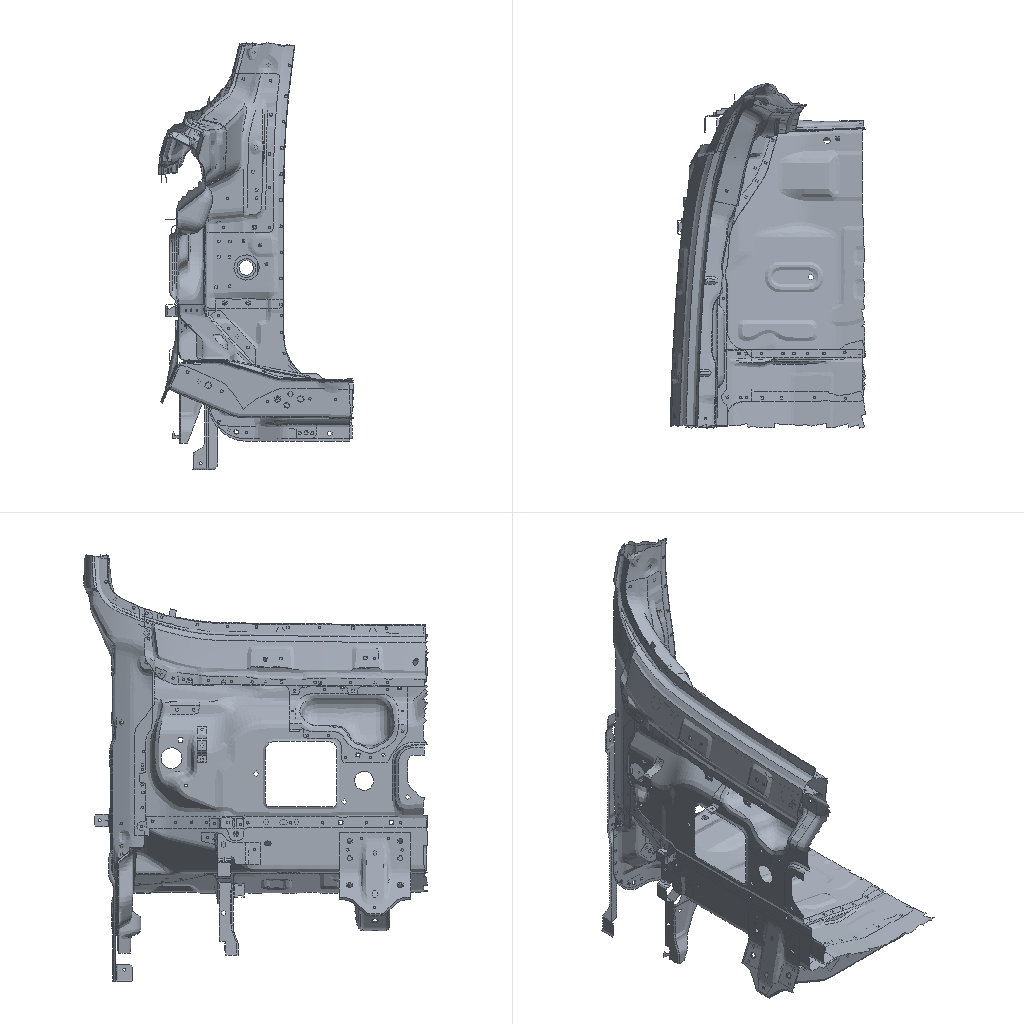Simulation study | nastran
Set-up summary:
category,name,step,type,value,unit,region
solver,nx_nastran
units,not stated in the deck,,not stated
analysis,deck,,static,static
analysis,solution,,SOL,101
load_step,SUBCASE 1,1,SUBCASE,SPC=6 LOAD=1
load_step,SUBCASE 2,2,SUBCASE,SPC=6 LOAD=2
load_step,SUBCASE 3,3,SUBCASE,SPC=6 LOAD=3
load_step,SUBCASE 4,4,SUBCASE,SPC=6 LOAD=4
load_step,requested,,,4
mesh,nodes,,,34995
mesh,elements,,,31458
element_type,CHEXA,,unverified,261
element_type,CONM2,,mass,1
element_type,CQUAD4,,shell,29179
element_type,CTRIA3,,shell,2278
load,load commands in deck,,count,4
bc,support commands in deck,,count,604
check,setup vs results,,match,"every grid point's frame and coordinates and every element id; grid points of CHEXA, CQUAD4, CTRIA3 elements"
Nastran input file, long lists of numbers shortened:
$$------------------------------------------------------------------------------$
$$                                                                              $
$$ NASTRAN Input Deck Generated by HyperMesh Version  : 9.0b121                 $
$$ Generated using HyperMesh-Nastran Template Version : 9.0b121
$$                                                                              $
$$   Template:  general                                                         $
$$                                                                              $
$$------------------------------------------------------------------------------$
$$------------------------------------------------------------------------------$
$$                      Executive Control Cards                                 $
$$------------------------------------------------------------------------------$
SOL 101
CEND
$$------------------------------------------------------------------------------$
$$                      Case Control Cards                                      $
$$------------------------------------------------------------------------------$
  DISPLACEMENT = ALL
  STRESS = ALL
  STRAIN = ALL
$
$HMNAME LOADSTEP               1"Step_X2g"
SUBCASE       1
  LABEL=         Step_X2g
  SPC =        6
  LOAD =        1
$
$HMNAME LOADSTEP               2"Step_Y2g"
SUBCASE       2
  LABEL=         Step_Y2g
  SPC =        6
  LOAD =        2
$
$HMNAME LOADSTEP               3"Step_Z2g"
SUBCASE       3
  LABEL=         Step_Z2g
  SPC =        6
  LOAD =        3
$
$HMNAME LOADSTEP               4"Step_Z-4g"
SUBCASE       4
  LABEL=         Step_Z-4g
  SPC =        6
  LOAD =        4
$$------------------------------------------------------------------------------$
$$                      Bulk Data Cards                                         $
$$------------------------------------------------------------------------------$
BEGIN BULK
PARAM,POST,-1
$$
$$  GRID Data
$$
GRID          26        -1028.271013.195590.4056
GRID          27        -1030.611013.072584.7464
$ (34993 more lines like these left out)
$$
$$  SPOINT Data
$$
$
$  CONM2 Elements
$
CONM2    103454184122189       00.0035380.0     0.0     0.0
$
$HMMOVE 84022691
$        1034541
$
$$
$$------------------------------------------------------------------------------$
$$             Group Definitions                                                $
$$------------------------------------------------------------------------------$
$
$ RBE2 Elements - Single dependent node
$
RBE2      346605 3700210  123456 3696816
RBE2      346606 3700211  123456 3696815
$ (12 more lines like these left out)
$
$HMMOVE 57005014
$         346605THRU      346608  346610THRU      346612  346614THRU      346620
$
$$
$$ RBE2 Elements - Multiple dependent nodes
$$
RBE2      346604 3700209  123456 3696817 3696994
RBE2      346609 3700214  123456 3696627 3696628
$ (85 more lines like these left out)
$
$HMMOVE 57005014
$         346604  346609  346613  346621  346623THRU      346624  346631THRU
$         346634  346871 1034566 1034540 1034567THRU     1034569
$
$
$  RBE3 Elements
$
RBE3      326301         3755368  1234560.294793     123 37252000.075522+
+            123 37251970.128418     123 37251930.501266     123 3725196
RBE3      326302         3755369  1234560.049321     123 37252000.318302+
+            123 37251970.547536     123 37251930.084841     123 3725196
$ (4172 more lines like these left out)
$
$HMMOVE 57005012
$         326301THRU      326304  326306THRU      326313  326315THRU      326322
$         326324THRU      326331  326333THRU      326336  326427THRU      326430
$ (108 more lines like these left out)
CTRIA3    170068       1   86527   86519   86520
CTRIA3    170076       1   86552   86587   86551
$ (2276 more lines like these left out)
$
$HMMOVE       17
$         170068  170076  170079  170087  170090  170093  170098  170103  170118
$         170125THRU      170126  170133  170159  170174  170181  170184  170189
$ (289 more lines like these left out)
CQUAD4    170067       1   86518   86519   86527   86528
CQUAD4    170069       1   86525   86524   86516   86517
$ (29177 more lines like these left out)
$
$HMMOVE       17
$         170067  170069THRU      170075  170077THRU      170078  170080THRU
$         170086  170088THRU      170089  170091THRU      170092  170094THRU
$ (867 more lines like these left out)
CHEXA     326305      10 3755368 3755369 3755370 3755371 3755372 3755373+
+        3755374 3755375
CHEXA     326314      10 3755377 3755380 3755379 3755378 3755381 3755384+
+        3755383 3755382
$ (518 more lines like these left out)
$
$HMMOVE 57005011
$         326305  326314  326323  326332  326431  326440  326449  326458  326467
$         326476  326593  326602  326611  326620  326629  326638  326647  326656
$ (140 more lines like these left out)
PSHELL         3       11.8            1               1
$
$HMNAME PROP                   4"100" 4
$HWCOLOR PROP                  4       3
PSHELL         4       11.0            1               1
$
$HMNAME PROP                   5"150" 4
$HWCOLOR PROP                  5       3
PSHELL         5       11.5            1               1
$
$HMNAME PROP                   6"250" 4
$HWCOLOR PROP                  6       3
PSHELL         6       12.5            1               1
$
$HMNAME PROP                   7"200" 4
$HWCOLOR PROP                  7       3
PSHELL         7       12.0            1               1
$
$HMNAME PROP                   2"120" 4
$HWCOLOR PROP                  2       3
PSHELL         2       11.2            1               1
$
$
$
$HMNAME PROP                   1"80" 4
$HWCOLOR PROP                  1       3
PSHELL         1       10.8            1               1
$$
$$  PSOLID Data
$
$HMNAME PROP                  10"spot" 5
$HWCOLOR PROP                 10       3
PSOLID        10       1
$$
$$------------------------------------------------------------------------------$
$$                      Material Definition Cards                               $
$$------------------------------------------------------------------------------$
$$--------------------------------------------------------------
$$ HYPERMESH TAGS
$$--------------------------------------------------------------
$$BEGIN TAGS
$$END TAGS
$$
$$  MAT1 Data
$
$HMNAME MAT                    1"steel" "MAT1"
$HWCOLOR MAT                   1       3
MAT1           1210000.0        0.3     1.60E-08
$$
$$
$$
$$------------------------------------------------------------------------------$
$ (27 more lines like these left out)
GRAV           1        9800.0  2.0     0.0     0.0
$$
$HMNAME LOADCOL                2"Y2g"
$HWCOLOR LOADCOL               2       4
GRAV           2        9800.0  0.0     2.0     0.0
$$
$HMNAME LOADCOL                3"Z2g"
$HWCOLOR LOADCOL               3       5
GRAV           3        9800.0  0.0     0.0     2.0
$$
$HMNAME LOADCOL                4"Z-4g"
$HWCOLOR LOADCOL               4       6
GRAV           4        9800.0  0.0     0.0     -4.0
$$
$$
$$
$$
$$
$$
$$
$$
$$
$$
$$
$$  SPC Data
$$
SPC            6   88502  1234560.0
SPC            6   88503  1234560.0
SPC            6   88537  1234560.0
SPC            6   88619  1234560.0
$ (600 more lines like these left out)
$HMASSEM       1       3 REAR_FLOOR
$HMASSEM_IDS    5100301051004210510048115100211051004410510060105100971051006211
$HMASSEM_IDS    5100451151005613510064105100561251005311
$HMASSEM      28       4 5300010
$HMASSEM_IDS          17      19      20      22      24      25      26
$HMASSEM 5400200       6 sidebody_R
$HMASSEM_IDS    5400211054002120540040105400402054002010
$
ENDDATA
Results summary:
result,analysis,,,static
result,last_loadstep,,,4
result,primary field,,,displacements
result,max displacement,,,0.1528,model units